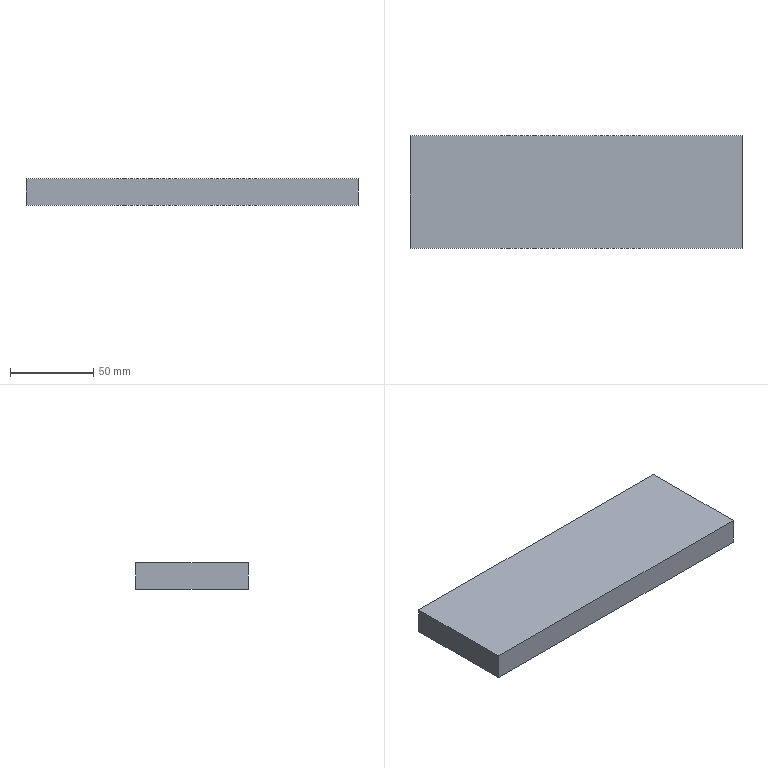Part | SolidWorks | features Extrusion 1 | 1 solid | 6 faces | box 200 x 68 x 16 mm | volume 217600 mm3 | plane 6
STEP:
#1=CARTESIAN_POINT('',(0.,68.,0.));
#2=VERTEX_POINT('',#1);
#3=CARTESIAN_POINT('',(0.,0.,0.));
#4=VERTEX_POINT('',#3);
#5=CARTESIAN_POINT('',(0.,0.,0.));
#6=DIRECTION('',(0.,-1.,0.));
#7=VECTOR('',#6,1000.);
#8=LINE('',#5,#7);
#9=EDGE_CURVE('',#2,#4,#8,.T.);
#10=ORIENTED_EDGE('',*,*,#9,.T.);
#11=CARTESIAN_POINT('',(0.,0.,16.));
#12=VERTEX_POINT('',#11);
#13=CARTESIAN_POINT('',(0.,0.,16.));
#14=DIRECTION('',(0.,0.,-1.));
#15=VECTOR('',#14,1000.);
#16=LINE('',#13,#15);
#17=EDGE_CURVE('',#12,#4,#16,.T.);
#18=ORIENTED_EDGE('',*,*,#17,.F.);
#19=CARTESIAN_POINT('',(0.,68.,16.));
#20=VERTEX_POINT('',#19);
#21=CARTESIAN_POINT('',(0.,0.,16.));
#22=DIRECTION('',(0.,-1.,0.));
#23=VECTOR('',#22,1000.);
#24=LINE('',#21,#23);
#25=EDGE_CURVE('',#20,#12,#24,.T.);
#26=ORIENTED_EDGE('',*,*,#25,.F.);
#27=CARTESIAN_POINT('',(0.,68.,16.));
#28=DIRECTION('',(0.,0.,-1.));
#29=VECTOR('',#28,1000.);
#30=LINE('',#27,#29);
#31=EDGE_CURVE('',#20,#2,#30,.T.);
#32=ORIENTED_EDGE('',*,*,#31,.T.);
#33=EDGE_LOOP('',(#10,#18,#26,#32));
#34=FACE_OUTER_BOUND('',#33,.T.);
#35=CARTESIAN_POINT('',(0.,0.,16.));
#36=DIRECTION('',(1.,0.,0.));
#37=DIRECTION('',(0.,0.,-1.));
#38=AXIS2_PLACEMENT_3D('',#35,#36,#37);
#39=PLANE('',#38);
#40=ADVANCED_FACE('',(#34),#39,.F.);
#41=CARTESIAN_POINT('',(200.,0.,0.));
#42=VERTEX_POINT('',#41);
#43=CARTESIAN_POINT('',(0.,0.,0.));
#44=DIRECTION('',(1.,0.,0.));
#45=VECTOR('',#44,1000.);
#46=LINE('',#43,#45);
#47=EDGE_CURVE('',#4,#42,#46,.T.);
#48=ORIENTED_EDGE('',*,*,#47,.T.);
#49=CARTESIAN_POINT('',(200.,0.,16.));
#50=VERTEX_POINT('',#49);
#51=CARTESIAN_POINT('',(200.,0.,16.));
#52=DIRECTION('',(0.,0.,-1.));
#53=VECTOR('',#52,1000.);
#54=LINE('',#51,#53);
#55=EDGE_CURVE('',#50,#42,#54,.T.);
#56=ORIENTED_EDGE('',*,*,#55,.F.);
#57=CARTESIAN_POINT('',(0.,0.,16.));
#58=DIRECTION('',(1.,0.,0.));
#59=VECTOR('',#58,1000.);
#60=LINE('',#57,#59);
#61=EDGE_CURVE('',#12,#50,#60,.T.);
#62=ORIENTED_EDGE('',*,*,#61,.F.);
#63=ORIENTED_EDGE('',*,*,#17,.T.);
#64=EDGE_LOOP('',(#48,#56,#62,#63));
#65=FACE_OUTER_BOUND('',#64,.T.);
#66=CARTESIAN_POINT('',(0.,0.,16.));
#67=DIRECTION('',(0.,1.,0.));
#68=DIRECTION('',(0.,0.,1.));
#69=AXIS2_PLACEMENT_3D('',#66,#67,#68);
#70=PLANE('',#69);
#71=ADVANCED_FACE('',(#65),#70,.F.);
#72=CARTESIAN_POINT('',(200.,68.,0.));
#73=VERTEX_POINT('',#72);
#74=CARTESIAN_POINT('',(200.,0.,0.));
#75=DIRECTION('',(0.,1.,0.));
#76=VECTOR('',#75,1000.);
#77=LINE('',#74,#76);
#78=EDGE_CURVE('',#42,#73,#77,.T.);
#79=ORIENTED_EDGE('',*,*,#78,.T.);
#80=CARTESIAN_POINT('',(200.,68.,16.));
#81=VERTEX_POINT('',#80);
#82=CARTESIAN_POINT('',(200.,68.,16.));
#83=DIRECTION('',(0.,0.,-1.));
#84=VECTOR('',#83,1000.);
#85=LINE('',#82,#84);
#86=EDGE_CURVE('',#81,#73,#85,.T.);
#87=ORIENTED_EDGE('',*,*,#86,.F.);
#88=CARTESIAN_POINT('',(200.,0.,16.));
#89=DIRECTION('',(0.,1.,0.));
#90=VECTOR('',#89,1000.);
#91=LINE('',#88,#90);
#92=EDGE_CURVE('',#50,#81,#91,.T.);
#93=ORIENTED_EDGE('',*,*,#92,.F.);
#94=ORIENTED_EDGE('',*,*,#55,.T.);
#95=EDGE_LOOP('',(#79,#87,#93,#94));
#96=FACE_OUTER_BOUND('',#95,.T.);
#97=CARTESIAN_POINT('',(200.,0.,16.));
#98=DIRECTION('',(-1.,0.,0.));
#99=DIRECTION('',(0.,0.,1.));
#100=AXIS2_PLACEMENT_3D('',#97,#98,#99);
#101=PLANE('',#100);
#102=ADVANCED_FACE('',(#96),#101,.F.);
#103=CARTESIAN_POINT('',(0.,68.,0.));
#104=DIRECTION('',(-1.,0.,0.));
#105=VECTOR('',#104,1000.);
#106=LINE('',#103,#105);
#107=EDGE_CURVE('',#73,#2,#106,.T.);
#108=ORIENTED_EDGE('',*,*,#107,.T.);
#109=ORIENTED_EDGE('',*,*,#31,.F.);
#110=CARTESIAN_POINT('',(0.,68.,16.));
#111=DIRECTION('',(-1.,0.,0.));
#112=VECTOR('',#111,1000.);
#113=LINE('',#110,#112);
#114=EDGE_CURVE('',#81,#20,#113,.T.);
#115=ORIENTED_EDGE('',*,*,#114,.F.);
#116=ORIENTED_EDGE('',*,*,#86,.T.);
#117=EDGE_LOOP('',(#108,#109,#115,#116));
#118=FACE_OUTER_BOUND('',#117,.T.);
#119=CARTESIAN_POINT('',(0.,68.,16.));
#120=DIRECTION('',(0.,-1.,0.));
#121=DIRECTION('',(0.,0.,-1.));
#122=AXIS2_PLACEMENT_3D('',#119,#120,#121);
#123=PLANE('',#122);
#124=ADVANCED_FACE('',(#118),#123,.F.);
#125=ORIENTED_EDGE('',*,*,#25,.T.);
#126=ORIENTED_EDGE('',*,*,#61,.T.);
#127=ORIENTED_EDGE('',*,*,#92,.T.);
#128=ORIENTED_EDGE('',*,*,#114,.T.);
#129=EDGE_LOOP('',(#125,#126,#127,#128));
#130=FACE_OUTER_BOUND('',#129,.T.);
#131=CARTESIAN_POINT('',(0.,0.,16.));
#132=DIRECTION('',(0.,0.,-1.));
#133=DIRECTION('',(-1.,0.,0.));
#134=AXIS2_PLACEMENT_3D('',#131,#132,#133);
#135=PLANE('',#134);
#136=ADVANCED_FACE('',(#130),#135,.F.);
#137=ORIENTED_EDGE('',*,*,#9,.F.);
#138=ORIENTED_EDGE('',*,*,#107,.F.);
#139=ORIENTED_EDGE('',*,*,#78,.F.);
#140=ORIENTED_EDGE('',*,*,#47,.F.);
#141=EDGE_LOOP('',(#137,#138,#139,#140));
#142=FACE_OUTER_BOUND('',#141,.T.);
#143=CARTESIAN_POINT('',(0.,0.,0.));
#144=DIRECTION('',(0.,0.,-1.));
#145=DIRECTION('',(-1.,0.,0.));
#146=AXIS2_PLACEMENT_3D('',#143,#144,#145);
#147=PLANE('',#146);
#148=ADVANCED_FACE('',(#142),#147,.T.);
#149=CLOSED_SHELL('',(#40,#71,#102,#124,#136,#148));
#150=MANIFOLD_SOLID_BREP('',#149);
#151=CARTESIAN_POINT('',(0.,0.,0.));
#152=DIRECTION('',(0.,0.,1.));
#153=DIRECTION('',(1.,0.,0.));
#154=AXIS2_PLACEMENT_3D('',#151,#152,#153);
#155=(LENGTH_UNIT()NAMED_UNIT(*)SI_UNIT(.MILLI.,.METRE.));
#156=UNCERTAINTY_MEASURE_WITH_UNIT(LENGTH_MEASURE(0.00001),#155,'','');
#157=(NAMED_UNIT(*)PLANE_ANGLE_UNIT()SI_UNIT($,.RADIAN.));
#158=(NAMED_UNIT(*)SI_UNIT($,.STERADIAN.)SOLID_ANGLE_UNIT());
#159=(GEOMETRIC_REPRESENTATION_CONTEXT(3)GLOBAL_UNCERTAINTY_ASSIGNED_CONTEXT((#156))GLOBAL_UNIT_ASSIGNED_CONTEXT((#155,#157,#158))REPRESENTATION_CONTEXT('',''));
#160=ADVANCED_BREP_SHAPE_REPRESENTATION('',(#150,#154),#159);